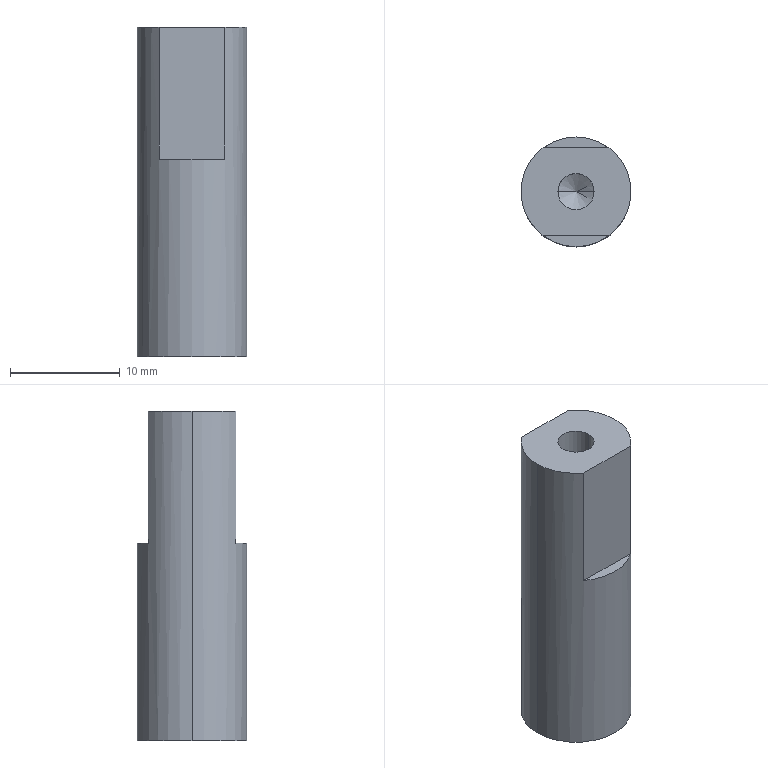Part | STEP file | 2073 Stop shaft | 1 solid | 16 faces | box 10 x 10 x 30 mm | volume 2056 mm3 | cylinder 6 | plane 6 | cone 4 | commonest cylinder face diameters 3.3 x4 10 x2
STEP:
#1=CARTESIAN_POINT('',(0.,0.,0.));
#2=DIRECTION('',(0.,0.,1.));
#3=DIRECTION('',(1.,0.,0.));
#4=AXIS2_PLACEMENT_3D('',#1,#2,#3);
#5=CARTESIAN_POINT('',(-1.65,0.,11.5));
#6=VERTEX_POINT('',#5);
#7=CARTESIAN_POINT('',(-1.65,0.,0.));
#8=VERTEX_POINT('',#7);
#9=CARTESIAN_POINT('',(-1.65,0.,0.));
#10=DIRECTION('',(0.,0.,-1.));
#11=VECTOR('',#10,1.);
#12=LINE('',#9,#11);
#13=CARTESIAN_POINT('',(0.,0.,0.));
#14=DIRECTION('',(0.,0.,-1.));
#15=DIRECTION('',(-1.,0.,0.));
#16=AXIS2_PLACEMENT_3D('',#13,#14,#15);
#17=CYLINDRICAL_SURFACE('',#16,1.65);
#18=CARTESIAN_POINT('',(6.283,0.));
#19=DIRECTION('',(0.,1.));
#20=VECTOR('',#19,1.);
#21=LINE('',#18,#20);
#22=(GEOMETRIC_REPRESENTATION_CONTEXT(2)PARAMETRIC_REPRESENTATION_CONTEXT()REPRESENTATION_CONTEXT('',''));
#23=DEFINITIONAL_REPRESENTATION('',(#21),#22);
#24=PCURVE('',#17,#23);
#25=CARTESIAN_POINT('',(0.,0.,0.));
#26=DIRECTION('',(0.,0.,-1.));
#27=DIRECTION('',(-1.,0.,0.));
#28=AXIS2_PLACEMENT_3D('',#25,#26,#27);
#29=CYLINDRICAL_SURFACE('',#28,1.65);
#30=CARTESIAN_POINT('',(0.,0.));
#31=DIRECTION('',(0.,1.));
#32=VECTOR('',#31,1.);
#33=LINE('',#30,#32);
#34=(GEOMETRIC_REPRESENTATION_CONTEXT(2)PARAMETRIC_REPRESENTATION_CONTEXT()REPRESENTATION_CONTEXT('',''));
#35=DEFINITIONAL_REPRESENTATION('',(#33),#34);
#36=PCURVE('',#29,#35);
#37=SURFACE_CURVE('',#12,(#24,#36),.PCURVE_S1.);
#38=EDGE_CURVE('',#6,#8,#37,.T.);
#39=ORIENTED_EDGE('',*,*,#38,.T.);
#40=CARTESIAN_POINT('',(1.65,0.,0.));
#41=VERTEX_POINT('',#40);
#42=CARTESIAN_POINT('',(0.,0.,0.));
#43=DIRECTION('',(0.,0.,-1.));
#44=DIRECTION('',(-1.,0.,0.));
#45=AXIS2_PLACEMENT_3D('',#42,#43,#44);
#46=CIRCLE('',#45,1.65);
#47=CARTESIAN_POINT('',(0.,0.));
#48=DIRECTION('',(1.,0.));
#49=VECTOR('',#48,1.);
#50=LINE('',#47,#49);
#51=(GEOMETRIC_REPRESENTATION_CONTEXT(2)PARAMETRIC_REPRESENTATION_CONTEXT()REPRESENTATION_CONTEXT('',''));
#52=DEFINITIONAL_REPRESENTATION('',(#50),#51);
#53=PCURVE('',#17,#52);
#54=CARTESIAN_POINT('',(0.,0.,0.));
#55=DIRECTION('',(0.,0.,1.));
#56=DIRECTION('',(1.,0.,0.));
#57=AXIS2_PLACEMENT_3D('',#54,#55,#56);
#58=PLANE('',#57);
#59=CARTESIAN_POINT('',(-1.65,0.));
#60=CARTESIAN_POINT('',(-1.65,2.858));
#61=CARTESIAN_POINT('',(0.825,1.429));
#62=CARTESIAN_POINT('',(3.3,0.));
#63=CARTESIAN_POINT('',(0.825,-1.429));
#64=CARTESIAN_POINT('',(-1.65,-2.858));
#65=CARTESIAN_POINT('',(-1.65,0.));
#66=(BOUNDED_CURVE()B_SPLINE_CURVE(2,(#59,#60,#61,#62,#63,#64,#65),.UNSPECIFIED.,.T.,.F.)B_SPLINE_CURVE_WITH_KNOTS((1,2,2,2,2,1),(-2.094,0.,2.094,4.189,6.283,8.378),.UNSPECIFIED.)CURVE()GEOMETRIC_REPRESENTATION_ITEM()RATIONAL_B_SPLINE_CURVE((1.,0.5,1.,0.5,1.,0.5,1.))REPRESENTATION_ITEM(''));
#67=(GEOMETRIC_REPRESENTATION_CONTEXT(2)PARAMETRIC_REPRESENTATION_CONTEXT()REPRESENTATION_CONTEXT('',''));
#68=DEFINITIONAL_REPRESENTATION('',(#66),#67);
#69=PCURVE('',#58,#68);
#70=SURFACE_CURVE('',#46,(#53,#69),.PCURVE_S1.);
#71=EDGE_CURVE('',#41,#8,#70,.T.);
#72=ORIENTED_EDGE('',*,*,#71,.F.);
#73=CARTESIAN_POINT('',(1.65,0.,11.5));
#74=VERTEX_POINT('',#73);
#75=CARTESIAN_POINT('',(1.65,0.,0.));
#76=DIRECTION('',(0.,0.,-1.));
#77=VECTOR('',#76,1.);
#78=LINE('',#75,#77);
#79=CARTESIAN_POINT('',(3.142,0.));
#80=DIRECTION('',(0.,1.));
#81=VECTOR('',#80,1.);
#82=LINE('',#79,#81);
#83=(GEOMETRIC_REPRESENTATION_CONTEXT(2)PARAMETRIC_REPRESENTATION_CONTEXT()REPRESENTATION_CONTEXT('',''));
#84=DEFINITIONAL_REPRESENTATION('',(#82),#83);
#85=PCURVE('',#17,#84);
#86=CARTESIAN_POINT('',(3.142,0.));
#87=DIRECTION('',(0.,1.));
#88=VECTOR('',#87,1.);
#89=LINE('',#86,#88);
#90=(GEOMETRIC_REPRESENTATION_CONTEXT(2)PARAMETRIC_REPRESENTATION_CONTEXT()REPRESENTATION_CONTEXT('',''));
#91=DEFINITIONAL_REPRESENTATION('',(#89),#90);
#92=PCURVE('',#29,#91);
#93=SURFACE_CURVE('',#78,(#85,#92),.PCURVE_S1.);
#94=EDGE_CURVE('',#74,#41,#93,.T.);
#95=ORIENTED_EDGE('',*,*,#94,.F.);
#96=CARTESIAN_POINT('',(0.,0.,11.5));
#97=DIRECTION('',(0.,0.,-1.));
#98=DIRECTION('',(-1.,0.,0.));
#99=AXIS2_PLACEMENT_3D('',#96,#97,#98);
#100=CIRCLE('',#99,1.65);
#101=CARTESIAN_POINT('',(0.,-11.5));
#102=DIRECTION('',(1.,0.));
#103=VECTOR('',#102,1.);
#104=LINE('',#101,#103);
#105=(GEOMETRIC_REPRESENTATION_CONTEXT(2)PARAMETRIC_REPRESENTATION_CONTEXT()REPRESENTATION_CONTEXT('',''));
#106=DEFINITIONAL_REPRESENTATION('',(#104),#105);
#107=PCURVE('',#17,#106);
#108=CARTESIAN_POINT('',(0.,0.,11.5));
#109=DIRECTION('',(0.,0.,-1.));
#110=DIRECTION('',(-1.,0.,0.));
#111=AXIS2_PLACEMENT_3D('',#108,#109,#110);
#112=CONICAL_SURFACE('',#111,1.65,1.03);
#113=CARTESIAN_POINT('',(0.,0.));
#114=DIRECTION('',(1.,0.));
#115=VECTOR('',#114,1.);
#116=LINE('',#113,#115);
#117=(GEOMETRIC_REPRESENTATION_CONTEXT(2)PARAMETRIC_REPRESENTATION_CONTEXT()REPRESENTATION_CONTEXT('',''));
#118=DEFINITIONAL_REPRESENTATION('',(#116),#117);
#119=PCURVE('',#112,#118);
#120=SURFACE_CURVE('',#100,(#107,#119),.PCURVE_S1.);
#121=EDGE_CURVE('',#74,#6,#120,.T.);
#122=ORIENTED_EDGE('',*,*,#121,.T.);
#123=EDGE_LOOP('',(#39,#72,#95,#122));
#124=FACE_BOUND('',#123,.F.);
#125=ADVANCED_FACE('',(#124),#17,.F.);
#126=ORIENTED_EDGE('',*,*,#121,.F.);
#127=CARTESIAN_POINT('',(0.,0.,12.491));
#128=VERTEX_POINT('',#127);
#129=CARTESIAN_POINT('',(1.65,0.,11.5));
#130=DIRECTION('',(0.8572,0.,-0.515));
#131=VECTOR('',#130,1.);
#132=LINE('',#129,#131);
#133=CARTESIAN_POINT('',(3.142,0.));
#134=DIRECTION('',(0.,1.));
#135=VECTOR('',#134,1.);
#136=LINE('',#133,#135);
#137=(GEOMETRIC_REPRESENTATION_CONTEXT(2)PARAMETRIC_REPRESENTATION_CONTEXT()REPRESENTATION_CONTEXT('',''));
#138=DEFINITIONAL_REPRESENTATION('',(#136),#137);
#139=PCURVE('',#112,#138);
#140=CARTESIAN_POINT('',(0.,0.,11.5));
#141=DIRECTION('',(0.,0.,-1.));
#142=DIRECTION('',(-1.,0.,0.));
#143=AXIS2_PLACEMENT_3D('',#140,#141,#142);
#144=CONICAL_SURFACE('',#143,1.65,1.03);
#145=CARTESIAN_POINT('',(3.142,0.));
#146=DIRECTION('',(0.,1.));
#147=VECTOR('',#146,1.);
#148=LINE('',#145,#147);
#149=(GEOMETRIC_REPRESENTATION_CONTEXT(2)PARAMETRIC_REPRESENTATION_CONTEXT()REPRESENTATION_CONTEXT('',''));
#150=DEFINITIONAL_REPRESENTATION('',(#148),#149);
#151=PCURVE('',#144,#150);
#152=SURFACE_CURVE('',#132,(#139,#151),.PCURVE_S1.);
#153=EDGE_CURVE('',#128,#74,#152,.T.);
#154=ORIENTED_EDGE('',*,*,#153,.F.);
#155=CARTESIAN_POINT('',(-1.65,0.,11.5));
#156=DIRECTION('',(-0.8572,0.,-0.515));
#157=VECTOR('',#156,1.);
#158=LINE('',#155,#157);
#159=CARTESIAN_POINT('',(6.283,0.));
#160=DIRECTION('',(0.,1.));
#161=VECTOR('',#160,1.);
#162=LINE('',#159,#161);
#163=(GEOMETRIC_REPRESENTATION_CONTEXT(2)PARAMETRIC_REPRESENTATION_CONTEXT()REPRESENTATION_CONTEXT('',''));
#164=DEFINITIONAL_REPRESENTATION('',(#162),#163);
#165=PCURVE('',#112,#164);
#166=CARTESIAN_POINT('',(0.,0.));
#167=DIRECTION('',(0.,1.));
#168=VECTOR('',#167,1.);
#169=LINE('',#166,#168);
#170=(GEOMETRIC_REPRESENTATION_CONTEXT(2)PARAMETRIC_REPRESENTATION_CONTEXT()REPRESENTATION_CONTEXT('',''));
#171=DEFINITIONAL_REPRESENTATION('',(#169),#170);
#172=PCURVE('',#144,#171);
#173=SURFACE_CURVE('',#158,(#165,#172),.PCURVE_S1.);
#174=EDGE_CURVE('',#128,#6,#173,.T.);
#175=ORIENTED_EDGE('',*,*,#174,.T.);
#176=EDGE_LOOP('',(#126,#154,#175));
#177=FACE_BOUND('',#176,.F.);
#178=ADVANCED_FACE('',(#177),#112,.F.);
#179=CARTESIAN_POINT('',(1.65,0.,18.5));
#180=VERTEX_POINT('',#179);
#181=CARTESIAN_POINT('',(1.65,0.,30.));
#182=VERTEX_POINT('',#181);
#183=CARTESIAN_POINT('',(1.65,0.,30.));
#184=DIRECTION('',(0.,0.,1.));
#185=VECTOR('',#184,1.);
#186=LINE('',#183,#185);
#187=CARTESIAN_POINT('',(0.,0.,30.));
#188=DIRECTION('',(0.,0.,1.));
#189=DIRECTION('',(1.,0.,0.));
#190=AXIS2_PLACEMENT_3D('',#187,#188,#189);
#191=CYLINDRICAL_SURFACE('',#190,1.65);
#192=CARTESIAN_POINT('',(6.283,0.));
#193=DIRECTION('',(0.,1.));
#194=VECTOR('',#193,1.);
#195=LINE('',#192,#194);
#196=(GEOMETRIC_REPRESENTATION_CONTEXT(2)PARAMETRIC_REPRESENTATION_CONTEXT()REPRESENTATION_CONTEXT('',''));
#197=DEFINITIONAL_REPRESENTATION('',(#195),#196);
#198=PCURVE('',#191,#197);
#199=CARTESIAN_POINT('',(0.,0.,30.));
#200=DIRECTION('',(0.,0.,1.));
#201=DIRECTION('',(1.,0.,0.));
#202=AXIS2_PLACEMENT_3D('',#199,#200,#201);
#203=CYLINDRICAL_SURFACE('',#202,1.65);
#204=CARTESIAN_POINT('',(0.,0.));
#205=DIRECTION('',(0.,1.));
#206=VECTOR('',#205,1.);
#207=LINE('',#204,#206);
#208=(GEOMETRIC_REPRESENTATION_CONTEXT(2)PARAMETRIC_REPRESENTATION_CONTEXT()REPRESENTATION_CONTEXT('',''));
#209=DEFINITIONAL_REPRESENTATION('',(#207),#208);
#210=PCURVE('',#203,#209);
#211=SURFACE_CURVE('',#186,(#198,#210),.PCURVE_S1.);
#212=EDGE_CURVE('',#180,#182,#211,.T.);
#213=ORIENTED_EDGE('',*,*,#212,.T.);
#214=CARTESIAN_POINT('',(-1.65,0.,30.));
#215=VERTEX_POINT('',#214);
#216=CARTESIAN_POINT('',(0.,0.,30.));
#217=DIRECTION('',(0.,0.,1.));
#218=DIRECTION('',(1.,0.,0.));
#219=AXIS2_PLACEMENT_3D('',#216,#217,#218);
#220=CIRCLE('',#219,1.65);
#221=CARTESIAN_POINT('',(0.,0.));
#222=DIRECTION('',(1.,0.));
#223=VECTOR('',#222,1.);
#224=LINE('',#221,#223);
#225=(GEOMETRIC_REPRESENTATION_CONTEXT(2)PARAMETRIC_REPRESENTATION_CONTEXT()REPRESENTATION_CONTEXT('',''));
#226=DEFINITIONAL_REPRESENTATION('',(#224),#225);
#227=PCURVE('',#191,#226);
#228=CARTESIAN_POINT('',(0.,0.,30.));
#229=DIRECTION('',(0.,0.,1.));
#230=DIRECTION('',(1.,0.,0.));
#231=AXIS2_PLACEMENT_3D('',#228,#229,#230);
#232=PLANE('',#231);
#233=CARTESIAN_POINT('',(0.,0.));
#234=DIRECTION('',(1.,0.));
#235=AXIS2_PLACEMENT_2D('',#233,#234);
#236=CIRCLE('',#235,1.65);
#237=(GEOMETRIC_REPRESENTATION_CONTEXT(2)PARAMETRIC_REPRESENTATION_CONTEXT()REPRESENTATION_CONTEXT('',''));
#238=DEFINITIONAL_REPRESENTATION('',(#236),#237);
#239=PCURVE('',#232,#238);
#240=SURFACE_CURVE('',#220,(#227,#239),.PCURVE_S1.);
#241=EDGE_CURVE('',#215,#182,#240,.T.);
#242=ORIENTED_EDGE('',*,*,#241,.F.);
#243=CARTESIAN_POINT('',(-1.65,0.,18.5));
#244=VERTEX_POINT('',#243);
#245=CARTESIAN_POINT('',(-1.65,0.,30.));
#246=DIRECTION('',(0.,0.,1.));
#247=VECTOR('',#246,1.);
#248=LINE('',#245,#247);
#249=CARTESIAN_POINT('',(3.142,0.));
#250=DIRECTION('',(0.,1.));
#251=VECTOR('',#250,1.);
#252=LINE('',#249,#251);
#253=(GEOMETRIC_REPRESENTATION_CONTEXT(2)PARAMETRIC_REPRESENTATION_CONTEXT()REPRESENTATION_CONTEXT('',''));
#254=DEFINITIONAL_REPRESENTATION('',(#252),#253);
#255=PCURVE('',#191,#254);
#256=CARTESIAN_POINT('',(3.142,0.));
#257=DIRECTION('',(0.,1.));
#258=VECTOR('',#257,1.);
#259=LINE('',#256,#258);
#260=(GEOMETRIC_REPRESENTATION_CONTEXT(2)PARAMETRIC_REPRESENTATION_CONTEXT()REPRESENTATION_CONTEXT('',''));
#261=DEFINITIONAL_REPRESENTATION('',(#259),#260);
#262=PCURVE('',#203,#261);
#263=SURFACE_CURVE('',#248,(#255,#262),.PCURVE_S1.);
#264=EDGE_CURVE('',#244,#215,#263,.T.);
#265=ORIENTED_EDGE('',*,*,#264,.F.);
#266=CARTESIAN_POINT('',(0.,0.,18.5));
#267=DIRECTION('',(0.,0.,1.));
#268=DIRECTION('',(1.,0.,0.));
#269=AXIS2_PLACEMENT_3D('',#266,#267,#268);
#270=CIRCLE('',#269,1.65);
#271=CARTESIAN_POINT('',(0.,-11.5));
#272=DIRECTION('',(1.,0.));
#273=VECTOR('',#272,1.);
#274=LINE('',#271,#273);
#275=(GEOMETRIC_REPRESENTATION_CONTEXT(2)PARAMETRIC_REPRESENTATION_CONTEXT()REPRESENTATION_CONTEXT('',''));
#276=DEFINITIONAL_REPRESENTATION('',(#274),#275);
#277=PCURVE('',#191,#276);
#278=CARTESIAN_POINT('',(0.,0.,18.5));
#279=DIRECTION('',(0.,0.,1.));
#280=DIRECTION('',(1.,0.,0.));
#281=AXIS2_PLACEMENT_3D('',#278,#279,#280);
#282=CONICAL_SURFACE('',#281,1.65,1.03);
#283=CARTESIAN_POINT('',(0.,0.));
#284=DIRECTION('',(1.,0.));
#285=VECTOR('',#284,1.);
#286=LINE('',#283,#285);
#287=(GEOMETRIC_REPRESENTATION_CONTEXT(2)PARAMETRIC_REPRESENTATION_CONTEXT()REPRESENTATION_CONTEXT('',''));
#288=DEFINITIONAL_REPRESENTATION('',(#286),#287);
#289=PCURVE('',#282,#288);
#290=SURFACE_CURVE('',#270,(#277,#289),.PCURVE_S1.);
#291=EDGE_CURVE('',#244,#180,#290,.T.);
#292=ORIENTED_EDGE('',*,*,#291,.T.);
#293=EDGE_LOOP('',(#213,#242,#265,#292));
#294=FACE_BOUND('',#293,.F.);
#295=ADVANCED_FACE('',(#294),#191,.F.);
#296=ORIENTED_EDGE('',*,*,#291,.F.);
#297=CARTESIAN_POINT('',(0.,0.,17.509));
#298=VERTEX_POINT('',#297);
#299=CARTESIAN_POINT('',(-1.65,0.,18.5));
#300=DIRECTION('',(-0.8572,0.,0.515));
#301=VECTOR('',#300,1.);
#302=LINE('',#299,#301);
#303=CARTESIAN_POINT('',(3.142,0.));
#304=DIRECTION('',(0.,1.));
#305=VECTOR('',#304,1.);
#306=LINE('',#303,#305);
#307=(GEOMETRIC_REPRESENTATION_CONTEXT(2)PARAMETRIC_REPRESENTATION_CONTEXT()REPRESENTATION_CONTEXT('',''));
#308=DEFINITIONAL_REPRESENTATION('',(#306),#307);
#309=PCURVE('',#282,#308);
#310=CARTESIAN_POINT('',(0.,0.,18.5));
#311=DIRECTION('',(0.,0.,1.));
#312=DIRECTION('',(1.,0.,0.));
#313=AXIS2_PLACEMENT_3D('',#310,#311,#312);
#314=CONICAL_SURFACE('',#313,1.65,1.03);
#315=CARTESIAN_POINT('',(3.142,0.));
#316=DIRECTION('',(0.,1.));
#317=VECTOR('',#316,1.);
#318=LINE('',#315,#317);
#319=(GEOMETRIC_REPRESENTATION_CONTEXT(2)PARAMETRIC_REPRESENTATION_CONTEXT()REPRESENTATION_CONTEXT('',''));
#320=DEFINITIONAL_REPRESENTATION('',(#318),#319);
#321=PCURVE('',#314,#320);
#322=SURFACE_CURVE('',#302,(#309,#321),.PCURVE_S1.);
#323=EDGE_CURVE('',#298,#244,#322,.T.);
#324=ORIENTED_EDGE('',*,*,#323,.F.);
#325=CARTESIAN_POINT('',(1.65,0.,18.5));
#326=DIRECTION('',(0.8572,0.,0.515));
#327=VECTOR('',#326,1.);
#328=LINE('',#325,#327);
#329=CARTESIAN_POINT('',(6.283,-0.9914));
#330=CARTESIAN_POINT('',(6.283,-0.9764));
#331=CARTESIAN_POINT('',(6.283,-0.9464));
#332=CARTESIAN_POINT('',(6.283,-0.9013));
#333=CARTESIAN_POINT('',(6.283,-0.8562));
#334=CARTESIAN_POINT('',(6.283,-0.8112));
#335=CARTESIAN_POINT('',(6.283,-0.7661));
#336=CARTESIAN_POINT('',(6.283,-0.721));
#337=CARTESIAN_POINT('',(6.283,-0.676));
#338=CARTESIAN_POINT('',(6.283,-0.6309));
#339=CARTESIAN_POINT('',(6.283,-0.5858));
#340=CARTESIAN_POINT('',(6.283,-0.5408));
#341=CARTESIAN_POINT('',(6.283,-0.4957));
#342=CARTESIAN_POINT('',(6.283,-0.4506));
#343=CARTESIAN_POINT('',(6.283,-0.4056));
#344=CARTESIAN_POINT('',(6.283,-0.3605));
#345=CARTESIAN_POINT('',(6.283,-0.3155));
#346=CARTESIAN_POINT('',(6.283,-0.2704));
#347=CARTESIAN_POINT('',(6.283,-0.2253));
#348=CARTESIAN_POINT('',(6.283,-0.1803));
#349=CARTESIAN_POINT('',(6.283,-0.1352));
#350=CARTESIAN_POINT('',(6.283,-0.09013));
#351=CARTESIAN_POINT('',(6.283,-0.04506));
#352=CARTESIAN_POINT('',(6.283,-0.01502));
#353=CARTESIAN_POINT('',(6.283,0.));
#354=B_SPLINE_CURVE_WITH_KNOTS('',3,(#329,#330,#331,#332,#333,#334,#335,#336,#337,#338,#339,#340,#341,#342,#343,#344,#345,#346,#347,#348,#349,#350,#351,#352,#353),.UNSPECIFIED.,.F.,.F.,(4,1,1,1,1,1,1,1,1,1,1,1,1,1,1,1,1,1,1,1,1,1,4),(-1.925,-1.837,-1.75,-1.662,-1.575,-1.487,-1.4,-1.312,-1.225,-1.137,-1.05,-0.9625,-0.875,-0.7875,-0.7,-0.6125,-0.525,-0.4375,-0.35,-0.2625,-0.175,-0.0875,0.),.UNSPECIFIED.);
#355=(GEOMETRIC_REPRESENTATION_CONTEXT(2)PARAMETRIC_REPRESENTATION_CONTEXT()REPRESENTATION_CONTEXT('',''));
#356=DEFINITIONAL_REPRESENTATION('',(#354),#355);
#357=PCURVE('',#282,#356);
#358=CARTESIAN_POINT('',(0.,-0.9914));
#359=CARTESIAN_POINT('',(0.,-0.9764));
#360=CARTESIAN_POINT('',(0.,-0.9464));
#361=CARTESIAN_POINT('',(0.,-0.9013));
#362=CARTESIAN_POINT('',(0.,-0.8562));
#363=CARTESIAN_POINT('',(0.,-0.8112));
#364=CARTESIAN_POINT('',(0.,-0.7661));
#365=CARTESIAN_POINT('',(0.,-0.721));
#366=CARTESIAN_POINT('',(0.,-0.676));
#367=CARTESIAN_POINT('',(0.,-0.6309));
#368=CARTESIAN_POINT('',(0.,-0.5858));
#369=CARTESIAN_POINT('',(0.,-0.5408));
#370=CARTESIAN_POINT('',(0.,-0.4957));
#371=CARTESIAN_POINT('',(0.,-0.4506));
#372=CARTESIAN_POINT('',(0.,-0.4056));
#373=CARTESIAN_POINT('',(0.,-0.3605));
#374=CARTESIAN_POINT('',(0.,-0.3155));
#375=CARTESIAN_POINT('',(0.,-0.2704));
#376=CARTESIAN_POINT('',(0.,-0.2253));
#377=CARTESIAN_POINT('',(0.,-0.1803));
#378=CARTESIAN_POINT('',(0.,-0.1352));
#379=CARTESIAN_POINT('',(0.,-0.09013));
#380=CARTESIAN_POINT('',(0.,-0.04506));
#381=CARTESIAN_POINT('',(0.,-0.01502));
#382=CARTESIAN_POINT('',(0.,0.));
#383=B_SPLINE_CURVE_WITH_KNOTS('',3,(#358,#359,#360,#361,#362,#363,#364,#365,#366,#367,#368,#369,#370,#371,#372,#373,#374,#375,#376,#377,#378,#379,#380,#381,#382),.UNSPECIFIED.,.F.,.F.,(4,1,1,1,1,1,1,1,1,1,1,1,1,1,1,1,1,1,1,1,1,1,4),(-1.925,-1.837,-1.75,-1.662,-1.575,-1.487,-1.4,-1.312,-1.225,-1.137,-1.05,-0.9625,-0.875,-0.7875,-0.7,-0.6125,-0.525,-0.4375,-0.35,-0.2625,-0.175,-0.0875,0.),.UNSPECIFIED.);
#384=(GEOMETRIC_REPRESENTATION_CONTEXT(2)PARAMETRIC_REPRESENTATION_CONTEXT()REPRESENTATION_CONTEXT('',''));
#385=DEFINITIONAL_REPRESENTATION('',(#383),#384);
#386=PCURVE('',#314,#385);
#387=SURFACE_CURVE('',#328,(#357,#386),.PCURVE_S1.);
#388=EDGE_CURVE('',#298,#180,#387,.T.);
#389=ORIENTED_EDGE('',*,*,#388,.T.);
#390=EDGE_LOOP('',(#296,#324,#389));
#391=FACE_BOUND('',#390,.F.);
#392=ADVANCED_FACE('',(#391),#282,.F.);
#393=CARTESIAN_POINT('',(5.,0.,30.));
#394=VERTEX_POINT('',#393);
#395=CARTESIAN_POINT('',(3.,4.,30.));
#396=VERTEX_POINT('',#395);
#397=CARTESIAN_POINT('',(0.,0.,30.));
#398=DIRECTION('',(0.,0.,1.));
#399=DIRECTION('',(1.,0.,0.));
#400=AXIS2_PLACEMENT_3D('',#397,#398,#399);
#401=CIRCLE('',#400,5.);
#402=CARTESIAN_POINT('',(0.,0.,30.));
#403=DIRECTION('',(0.,0.,-1.));
#404=DIRECTION('',(-1.,0.,0.));
#405=AXIS2_PLACEMENT_3D('',#402,#403,#404);
#406=CYLINDRICAL_SURFACE('',#405,5.);
#407=CARTESIAN_POINT('',(3.142,0.));
#408=DIRECTION('',(-1.,0.));
#409=VECTOR('',#408,1.);
#410=LINE('',#407,#409);
#411=(GEOMETRIC_REPRESENTATION_CONTEXT(2)PARAMETRIC_REPRESENTATION_CONTEXT()REPRESENTATION_CONTEXT('',''));
#412=DEFINITIONAL_REPRESENTATION('',(#410),#411);
#413=PCURVE('',#406,#412);
#414=CARTESIAN_POINT('',(0.,0.));
#415=DIRECTION('',(1.,0.));
#416=AXIS2_PLACEMENT_2D('',#414,#415);
#417=CIRCLE('',#416,5.);
#418=(GEOMETRIC_REPRESENTATION_CONTEXT(2)PARAMETRIC_REPRESENTATION_CONTEXT()REPRESENTATION_CONTEXT('',''));
#419=DEFINITIONAL_REPRESENTATION('',(#417),#418);
#420=PCURVE('',#232,#419);
#421=SURFACE_CURVE('',#401,(#413,#420),.PCURVE_S1.);
#422=EDGE_CURVE('',#394,#396,#421,.T.);
#423=ORIENTED_EDGE('',*,*,#422,.F.);
#424=CARTESIAN_POINT('',(5.,0.,0.));
#425=VERTEX_POINT('',#424);
#426=CARTESIAN_POINT('',(5.,0.,30.));
#427=DIRECTION('',(0.,0.,-1.));
#428=VECTOR('',#427,1.);
#429=LINE('',#426,#428);
#430=CARTESIAN_POINT('',(3.142,0.));
#431=DIRECTION('',(0.,1.));
#432=VECTOR('',#431,1.);
#433=LINE('',#430,#432);
#434=(GEOMETRIC_REPRESENTATION_CONTEXT(2)PARAMETRIC_REPRESENTATION_CONTEXT()REPRESENTATION_CONTEXT('',''));
#435=DEFINITIONAL_REPRESENTATION('',(#433),#434);
#436=PCURVE('',#406,#435);
#437=CARTESIAN_POINT('',(0.,0.,30.));
#438=DIRECTION('',(0.,0.,-1.));
#439=DIRECTION('',(-1.,0.,0.));
#440=AXIS2_PLACEMENT_3D('',#437,#438,#439);
#441=CYLINDRICAL_SURFACE('',#440,5.);
#442=CARTESIAN_POINT('',(3.142,0.));
#443=DIRECTION('',(0.,1.));
#444=VECTOR('',#443,1.);
#445=LINE('',#442,#444);
#446=(GEOMETRIC_REPRESENTATION_CONTEXT(2)PARAMETRIC_REPRESENTATION_CONTEXT()REPRESENTATION_CONTEXT('',''));
#447=DEFINITIONAL_REPRESENTATION('',(#445),#446);
#448=PCURVE('',#441,#447);
#449=SURFACE_CURVE('',#429,(#436,#448),.PCURVE_S1.);
#450=EDGE_CURVE('',#394,#425,#449,.T.);
#451=ORIENTED_EDGE('',*,*,#450,.T.);
#452=CARTESIAN_POINT('',(-5.,0.,0.));
#453=VERTEX_POINT('',#452);
#454=CARTESIAN_POINT('',(0.,0.,0.));
#455=DIRECTION('',(0.,0.,1.));
#456=DIRECTION('',(1.,0.,0.));
#457=AXIS2_PLACEMENT_3D('',#454,#455,#456);
#458=CIRCLE('',#457,5.);
#459=CARTESIAN_POINT('',(3.142,30.));
#460=DIRECTION('',(-1.,0.));
#461=VECTOR('',#460,1.);
#462=LINE('',#459,#461);
#463=(GEOMETRIC_REPRESENTATION_CONTEXT(2)PARAMETRIC_REPRESENTATION_CONTEXT()REPRESENTATION_CONTEXT('',''));
#464=DEFINITIONAL_REPRESENTATION('',(#462),#463);
#465=PCURVE('',#406,#464);
#466=CARTESIAN_POINT('',(0.,0.));
#467=DIRECTION('',(1.,0.));
#468=AXIS2_PLACEMENT_2D('',#466,#467);
#469=CIRCLE('',#468,5.);
#470=(GEOMETRIC_REPRESENTATION_CONTEXT(2)PARAMETRIC_REPRESENTATION_CONTEXT()REPRESENTATION_CONTEXT('',''));
#471=DEFINITIONAL_REPRESENTATION('',(#469),#470);
#472=PCURVE('',#58,#471);
#473=SURFACE_CURVE('',#458,(#465,#472),.PCURVE_S1.);
#474=EDGE_CURVE('',#425,#453,#473,.T.);
#475=ORIENTED_EDGE('',*,*,#474,.T.);
#476=CARTESIAN_POINT('',(-5.,0.,30.));
#477=VERTEX_POINT('',#476);
#478=CARTESIAN_POINT('',(-5.,0.,30.));
#479=DIRECTION('',(0.,0.,-1.));
#480=VECTOR('',#479,1.);
#481=LINE('',#478,#480);
#482=CARTESIAN_POINT('',(0.,0.));
#483=DIRECTION('',(0.,1.));
#484=VECTOR('',#483,1.);
#485=LINE('',#482,#484);
#486=(GEOMETRIC_REPRESENTATION_CONTEXT(2)PARAMETRIC_REPRESENTATION_CONTEXT()REPRESENTATION_CONTEXT('',''));
#487=DEFINITIONAL_REPRESENTATION('',(#485),#486);
#488=PCURVE('',#406,#487);
#489=CARTESIAN_POINT('',(6.283,0.));
#490=DIRECTION('',(0.,1.));
#491=VECTOR('',#490,1.);
#492=LINE('',#489,#491);
#493=(GEOMETRIC_REPRESENTATION_CONTEXT(2)PARAMETRIC_REPRESENTATION_CONTEXT()REPRESENTATION_CONTEXT('',''));
#494=DEFINITIONAL_REPRESENTATION('',(#492),#493);
#495=PCURVE('',#441,#494);
#496=SURFACE_CURVE('',#481,(#488,#495),.PCURVE_S1.);
#497=EDGE_CURVE('',#477,#453,#496,.T.);
#498=ORIENTED_EDGE('',*,*,#497,.F.);
#499=CARTESIAN_POINT('',(-3.,4.,30.));
#500=VERTEX_POINT('',#499);
#501=CARTESIAN_POINT('',(0.,0.,30.));
#502=DIRECTION('',(0.,0.,1.));
#503=DIRECTION('',(1.,0.,0.));
#504=AXIS2_PLACEMENT_3D('',#501,#502,#503);
#505=CIRCLE('',#504,5.);
#506=CARTESIAN_POINT('',(3.142,0.));
#507=DIRECTION('',(-1.,0.));
#508=VECTOR('',#507,1.);
#509=LINE('',#506,#508);
#510=(GEOMETRIC_REPRESENTATION_CONTEXT(2)PARAMETRIC_REPRESENTATION_CONTEXT()REPRESENTATION_CONTEXT('',''));
#511=DEFINITIONAL_REPRESENTATION('',(#509),#510);
#512=PCURVE('',#406,#511);
#513=CARTESIAN_POINT('',(0.,0.));
#514=DIRECTION('',(1.,0.));
#515=AXIS2_PLACEMENT_2D('',#513,#514);
#516=CIRCLE('',#515,5.);
#517=(GEOMETRIC_REPRESENTATION_CONTEXT(2)PARAMETRIC_REPRESENTATION_CONTEXT()REPRESENTATION_CONTEXT('',''));
#518=DEFINITIONAL_REPRESENTATION('',(#516),#517);
#519=PCURVE('',#232,#518);
#520=SURFACE_CURVE('',#505,(#512,#519),.PCURVE_S1.);
#521=EDGE_CURVE('',#500,#477,#520,.T.);
#522=ORIENTED_EDGE('',*,*,#521,.F.);
#523=CARTESIAN_POINT('',(-3.,4.,18.));
#524=VERTEX_POINT('',#523);
#525=CARTESIAN_POINT('',(-3.,4.,30.));
#526=DIRECTION('',(0.,0.,-1.));
#527=VECTOR('',#526,1.);
#528=LINE('',#525,#527);
#529=CARTESIAN_POINT('',(0.9273,0.));
#530=DIRECTION('',(0.,1.));
#531=VECTOR('',#530,1.);
#532=LINE('',#529,#531);
#533=(GEOMETRIC_REPRESENTATION_CONTEXT(2)PARAMETRIC_REPRESENTATION_CONTEXT()REPRESENTATION_CONTEXT('',''));
#534=DEFINITIONAL_REPRESENTATION('',(#532),#533);
#535=PCURVE('',#406,#534);
#536=CARTESIAN_POINT('',(-6.568,4.,18.));
#537=DIRECTION('',(0.,-1.,0.));
#538=DIRECTION('',(0.,0.,-1.));
#539=AXIS2_PLACEMENT_3D('',#536,#537,#538);
#540=PLANE('',#539);
#541=CARTESIAN_POINT('',(-12.,3.568));
#542=DIRECTION('',(1.,0.));
#543=VECTOR('',#542,1.);
#544=LINE('',#541,#543);
#545=(GEOMETRIC_REPRESENTATION_CONTEXT(2)PARAMETRIC_REPRESENTATION_CONTEXT()REPRESENTATION_CONTEXT('',''));
#546=DEFINITIONAL_REPRESENTATION('',(#544),#545);
#547=PCURVE('',#540,#546);
#548=SURFACE_CURVE('',#528,(#535,#547),.PCURVE_S1.);
#549=EDGE_CURVE('',#500,#524,#548,.T.);
#550=ORIENTED_EDGE('',*,*,#549,.T.);
#551=CARTESIAN_POINT('',(3.,4.,18.));
#552=VERTEX_POINT('',#551);
#553=CARTESIAN_POINT('',(0.,0.,18.));
#554=DIRECTION('',(0.,0.,1.));
#555=DIRECTION('',(1.,0.,0.));
#556=AXIS2_PLACEMENT_3D('',#553,#554,#555);
#557=CIRCLE('',#556,5.);
#558=CARTESIAN_POINT('',(3.142,12.));
#559=DIRECTION('',(-1.,0.));
#560=VECTOR('',#559,1.);
#561=LINE('',#558,#560);
#562=(GEOMETRIC_REPRESENTATION_CONTEXT(2)PARAMETRIC_REPRESENTATION_CONTEXT()REPRESENTATION_CONTEXT('',''));
#563=DEFINITIONAL_REPRESENTATION('',(#561),#562);
#564=PCURVE('',#406,#563);
#565=CARTESIAN_POINT('',(0.,0.,18.));
#566=DIRECTION('',(0.,0.,1.));
#567=DIRECTION('',(1.,0.,0.));
#568=AXIS2_PLACEMENT_3D('',#565,#566,#567);
#569=PLANE('',#568);
#570=CARTESIAN_POINT('',(0.,0.));
#571=DIRECTION('',(1.,0.));
#572=AXIS2_PLACEMENT_2D('',#570,#571);
#573=CIRCLE('',#572,5.);
#574=(GEOMETRIC_REPRESENTATION_CONTEXT(2)PARAMETRIC_REPRESENTATION_CONTEXT()REPRESENTATION_CONTEXT('',''));
#575=DEFINITIONAL_REPRESENTATION('',(#573),#574);
#576=PCURVE('',#569,#575);
#577=SURFACE_CURVE('',#557,(#564,#576),.PCURVE_S1.);
#578=EDGE_CURVE('',#552,#524,#577,.T.);
#579=ORIENTED_EDGE('',*,*,#578,.F.);
#580=CARTESIAN_POINT('',(3.,4.,30.));
#581=DIRECTION('',(0.,0.,1.));
#582=VECTOR('',#581,1.);
#583=LINE('',#580,#582);
#584=CARTESIAN_POINT('',(2.214,0.));
#585=DIRECTION('',(0.,-1.));
#586=VECTOR('',#585,1.);
#587=LINE('',#584,#586);
#588=(GEOMETRIC_REPRESENTATION_CONTEXT(2)PARAMETRIC_REPRESENTATION_CONTEXT()REPRESENTATION_CONTEXT('',''));
#589=DEFINITIONAL_REPRESENTATION('',(#587),#588);
#590=PCURVE('',#406,#589);
#591=CARTESIAN_POINT('',(-12.,9.568));
#592=DIRECTION('',(-1.,0.));
#593=VECTOR('',#592,1.);
#594=LINE('',#591,#593);
#595=(GEOMETRIC_REPRESENTATION_CONTEXT(2)PARAMETRIC_REPRESENTATION_CONTEXT()REPRESENTATION_CONTEXT('',''));
#596=DEFINITIONAL_REPRESENTATION('',(#594),#595);
#597=PCURVE('',#540,#596);
#598=SURFACE_CURVE('',#583,(#590,#597),.PCURVE_S1.);
#599=EDGE_CURVE('',#552,#396,#598,.T.);
#600=ORIENTED_EDGE('',*,*,#599,.T.);
#601=EDGE_LOOP('',(#423,#451,#475,#498,#522,#550,#579,#600));
#602=FACE_BOUND('',#601,.T.);
#603=ADVANCED_FACE('',(#602),#406,.T.);
#604=ORIENTED_EDGE('',*,*,#450,.F.);
#605=CARTESIAN_POINT('',(3.,-4.,30.));
#606=VERTEX_POINT('',#605);
#607=CARTESIAN_POINT('',(0.,0.,30.));
#608=DIRECTION('',(0.,0.,1.));
#609=DIRECTION('',(1.,0.,0.));
#610=AXIS2_PLACEMENT_3D('',#607,#608,#609);
#611=CIRCLE('',#610,5.);
#612=CARTESIAN_POINT('',(9.425,0.));
#613=DIRECTION('',(-1.,0.));
#614=VECTOR('',#613,1.);
#615=LINE('',#612,#614);
#616=(GEOMETRIC_REPRESENTATION_CONTEXT(2)PARAMETRIC_REPRESENTATION_CONTEXT()REPRESENTATION_CONTEXT('',''));
#617=DEFINITIONAL_REPRESENTATION('',(#615),#616);
#618=PCURVE('',#441,#617);
#619=CARTESIAN_POINT('',(0.,0.));
#620=DIRECTION('',(1.,0.));
#621=AXIS2_PLACEMENT_2D('',#619,#620);
#622=CIRCLE('',#621,5.);
#623=(GEOMETRIC_REPRESENTATION_CONTEXT(2)PARAMETRIC_REPRESENTATION_CONTEXT()REPRESENTATION_CONTEXT('',''));
#624=DEFINITIONAL_REPRESENTATION('',(#622),#623);
#625=PCURVE('',#232,#624);
#626=SURFACE_CURVE('',#611,(#618,#625),.PCURVE_S1.);
#627=EDGE_CURVE('',#606,#394,#626,.T.);
#628=ORIENTED_EDGE('',*,*,#627,.F.);
#629=CARTESIAN_POINT('',(3.,-4.,18.));
#630=VERTEX_POINT('',#629);
#631=CARTESIAN_POINT('',(3.,-4.,30.));
#632=DIRECTION('',(0.,0.,-1.));
#633=VECTOR('',#632,1.);
#634=LINE('',#631,#633);
#635=CARTESIAN_POINT('',(4.069,0.));
#636=DIRECTION('',(0.,1.));
#637=VECTOR('',#636,1.);
#638=LINE('',#635,#637);
#639=(GEOMETRIC_REPRESENTATION_CONTEXT(2)PARAMETRIC_REPRESENTATION_CONTEXT()REPRESENTATION_CONTEXT('',''));
#640=DEFINITIONAL_REPRESENTATION('',(#638),#639);
#641=PCURVE('',#441,#640);
#642=CARTESIAN_POINT('',(-6.782,-4.,18.));
#643=DIRECTION('',(0.,1.,0.));
#644=DIRECTION('',(0.,0.,1.));
#645=AXIS2_PLACEMENT_3D('',#642,#643,#644);
#646=PLANE('',#645);
#647=CARTESIAN_POINT('',(12.,9.782));
#648=DIRECTION('',(-1.,0.));
#649=VECTOR('',#648,1.);
#650=LINE('',#647,#649);
#651=(GEOMETRIC_REPRESENTATION_CONTEXT(2)PARAMETRIC_REPRESENTATION_CONTEXT()REPRESENTATION_CONTEXT('',''));
#652=DEFINITIONAL_REPRESENTATION('',(#650),#651);
#653=PCURVE('',#646,#652);
#654=SURFACE_CURVE('',#634,(#641,#653),.PCURVE_S1.);
#655=EDGE_CURVE('',#606,#630,#654,.T.);
#656=ORIENTED_EDGE('',*,*,#655,.T.);
#657=CARTESIAN_POINT('',(-3.,-4.,18.));
#658=VERTEX_POINT('',#657);
#659=CARTESIAN_POINT('',(0.,0.,18.));
#660=DIRECTION('',(0.,0.,1.));
#661=DIRECTION('',(1.,0.,0.));
#662=AXIS2_PLACEMENT_3D('',#659,#660,#661);
#663=CIRCLE('',#662,5.);
#664=CARTESIAN_POINT('',(9.425,12.));
#665=DIRECTION('',(-1.,0.));
#666=VECTOR('',#665,1.);
#667=LINE('',#664,#666);
#668=(GEOMETRIC_REPRESENTATION_CONTEXT(2)PARAMETRIC_REPRESENTATION_CONTEXT()REPRESENTATION_CONTEXT('',''));
#669=DEFINITIONAL_REPRESENTATION('',(#667),#668);
#670=PCURVE('',#441,#669);
#671=CARTESIAN_POINT('',(0.,0.,18.));
#672=DIRECTION('',(0.,0.,1.));
#673=DIRECTION('',(1.,0.,0.));
#674=AXIS2_PLACEMENT_3D('',#671,#672,#673);
#675=PLANE('',#674);
#676=CARTESIAN_POINT('',(0.,0.));
#677=DIRECTION('',(1.,0.));
#678=AXIS2_PLACEMENT_2D('',#676,#677);
#679=CIRCLE('',#678,5.);
#680=(GEOMETRIC_REPRESENTATION_CONTEXT(2)PARAMETRIC_REPRESENTATION_CONTEXT()REPRESENTATION_CONTEXT('',''));
#681=DEFINITIONAL_REPRESENTATION('',(#679),#680);
#682=PCURVE('',#675,#681);
#683=SURFACE_CURVE('',#663,(#670,#682),.PCURVE_S1.);
#684=EDGE_CURVE('',#658,#630,#683,.T.);
#685=ORIENTED_EDGE('',*,*,#684,.F.);
#686=CARTESIAN_POINT('',(-3.,-4.,30.));
#687=VERTEX_POINT('',#686);
#688=CARTESIAN_POINT('',(-3.,-4.,30.));
#689=DIRECTION('',(0.,0.,1.));
#690=VECTOR('',#689,1.);
#691=LINE('',#688,#690);
#692=CARTESIAN_POINT('',(5.356,0.));
#693=DIRECTION('',(0.,-1.));
#694=VECTOR('',#693,1.);
#695=LINE('',#692,#694);
#696=(GEOMETRIC_REPRESENTATION_CONTEXT(2)PARAMETRIC_REPRESENTATION_CONTEXT()REPRESENTATION_CONTEXT('',''));
#697=DEFINITIONAL_REPRESENTATION('',(#695),#696);
#698=PCURVE('',#441,#697);
#699=CARTESIAN_POINT('',(12.,3.782));
#700=DIRECTION('',(1.,0.));
#701=VECTOR('',#700,1.);
#702=LINE('',#699,#701);
#703=(GEOMETRIC_REPRESENTATION_CONTEXT(2)PARAMETRIC_REPRESENTATION_CONTEXT()REPRESENTATION_CONTEXT('',''));
#704=DEFINITIONAL_REPRESENTATION('',(#702),#703);
#705=PCURVE('',#646,#704);
#706=SURFACE_CURVE('',#691,(#698,#705),.PCURVE_S1.);
#707=EDGE_CURVE('',#658,#687,#706,.T.);
#708=ORIENTED_EDGE('',*,*,#707,.T.);
#709=CARTESIAN_POINT('',(0.,0.,30.));
#710=DIRECTION('',(0.,0.,1.));
#711=DIRECTION('',(1.,0.,0.));
#712=AXIS2_PLACEMENT_3D('',#709,#710,#711);
#713=CIRCLE('',#712,5.);
#714=CARTESIAN_POINT('',(9.425,0.));
#715=DIRECTION('',(-1.,0.));
#716=VECTOR('',#715,1.);
#717=LINE('',#714,#716);
#718=(GEOMETRIC_REPRESENTATION_CONTEXT(2)PARAMETRIC_REPRESENTATION_CONTEXT()REPRESENTATION_CONTEXT('',''));
#719=DEFINITIONAL_REPRESENTATION('',(#717),#718);
#720=PCURVE('',#441,#719);
#721=CARTESIAN_POINT('',(0.,0.));
#722=DIRECTION('',(1.,0.));
#723=AXIS2_PLACEMENT_2D('',#721,#722);
#724=CIRCLE('',#723,5.);
#725=(GEOMETRIC_REPRESENTATION_CONTEXT(2)PARAMETRIC_REPRESENTATION_CONTEXT()REPRESENTATION_CONTEXT('',''));
#726=DEFINITIONAL_REPRESENTATION('',(#724),#725);
#727=PCURVE('',#232,#726);
#728=SURFACE_CURVE('',#713,(#720,#727),.PCURVE_S1.);
#729=EDGE_CURVE('',#477,#687,#728,.T.);
#730=ORIENTED_EDGE('',*,*,#729,.F.);
#731=ORIENTED_EDGE('',*,*,#497,.T.);
#732=CARTESIAN_POINT('',(0.,0.,0.));
#733=DIRECTION('',(0.,0.,1.));
#734=DIRECTION('',(1.,0.,0.));
#735=AXIS2_PLACEMENT_3D('',#732,#733,#734);
#736=CIRCLE('',#735,5.);
#737=CARTESIAN_POINT('',(9.425,30.));
#738=DIRECTION('',(-1.,0.));
#739=VECTOR('',#738,1.);
#740=LINE('',#737,#739);
#741=(GEOMETRIC_REPRESENTATION_CONTEXT(2)PARAMETRIC_REPRESENTATION_CONTEXT()REPRESENTATION_CONTEXT('',''));
#742=DEFINITIONAL_REPRESENTATION('',(#740),#741);
#743=PCURVE('',#441,#742);
#744=CARTESIAN_POINT('',(0.,0.));
#745=DIRECTION('',(1.,0.));
#746=AXIS2_PLACEMENT_2D('',#744,#745);
#747=CIRCLE('',#746,5.);
#748=(GEOMETRIC_REPRESENTATION_CONTEXT(2)PARAMETRIC_REPRESENTATION_CONTEXT()REPRESENTATION_CONTEXT('',''));
#749=DEFINITIONAL_REPRESENTATION('',(#747),#748);
#750=PCURVE('',#58,#749);
#751=SURFACE_CURVE('',#736,(#743,#750),.PCURVE_S1.);
#752=EDGE_CURVE('',#453,#425,#751,.T.);
#753=ORIENTED_EDGE('',*,*,#752,.T.);
#754=EDGE_LOOP('',(#604,#628,#656,#685,#708,#730,#731,#753));
#755=FACE_BOUND('',#754,.T.);
#756=ADVANCED_FACE('',(#755),#441,.T.);
#757=CARTESIAN_POINT('',(0.,-4.,30.));
#758=DIRECTION('',(-1.,0.,0.));
#759=VECTOR('',#758,1.);
#760=LINE('',#757,#759);
#761=CARTESIAN_POINT('',(0.,-4.));
#762=DIRECTION('',(-1.,0.));
#763=VECTOR('',#762,1.);
#764=LINE('',#761,#763);
#765=(GEOMETRIC_REPRESENTATION_CONTEXT(2)PARAMETRIC_REPRESENTATION_CONTEXT()REPRESENTATION_CONTEXT('',''));
#766=DEFINITIONAL_REPRESENTATION('',(#764),#765);
#767=PCURVE('',#232,#766);
#768=CARTESIAN_POINT('',(12.,6.782));
#769=DIRECTION('',(0.,-1.));
#770=VECTOR('',#769,1.);
#771=LINE('',#768,#770);
#772=(GEOMETRIC_REPRESENTATION_CONTEXT(2)PARAMETRIC_REPRESENTATION_CONTEXT()REPRESENTATION_CONTEXT('',''));
#773=DEFINITIONAL_REPRESENTATION('',(#771),#772);
#774=PCURVE('',#646,#773);
#775=SURFACE_CURVE('',#760,(#767,#774),.PCURVE_S1.);
#776=EDGE_CURVE('',#606,#687,#775,.T.);
#777=ORIENTED_EDGE('',*,*,#776,.F.);
#778=ORIENTED_EDGE('',*,*,#627,.T.);
#779=ORIENTED_EDGE('',*,*,#422,.T.);
#780=CARTESIAN_POINT('',(0.,4.,30.));
#781=DIRECTION('',(1.,0.,0.));
#782=VECTOR('',#781,1.);
#783=LINE('',#780,#782);
#784=CARTESIAN_POINT('',(0.,4.));
#785=DIRECTION('',(1.,0.));
#786=VECTOR('',#785,1.);
#787=LINE('',#784,#786);
#788=(GEOMETRIC_REPRESENTATION_CONTEXT(2)PARAMETRIC_REPRESENTATION_CONTEXT()REPRESENTATION_CONTEXT('',''));
#789=DEFINITIONAL_REPRESENTATION('',(#787),#788);
#790=PCURVE('',#232,#789);
#791=CARTESIAN_POINT('',(-12.,6.568));
#792=DIRECTION('',(0.,1.));
#793=VECTOR('',#792,1.);
#794=LINE('',#791,#793);
#795=(GEOMETRIC_REPRESENTATION_CONTEXT(2)PARAMETRIC_REPRESENTATION_CONTEXT()REPRESENTATION_CONTEXT('',''));
#796=DEFINITIONAL_REPRESENTATION('',(#794),#795);
#797=PCURVE('',#540,#796);
#798=SURFACE_CURVE('',#783,(#790,#797),.PCURVE_S1.);
#799=EDGE_CURVE('',#500,#396,#798,.T.);
#800=ORIENTED_EDGE('',*,*,#799,.F.);
#801=ORIENTED_EDGE('',*,*,#521,.T.);
#802=ORIENTED_EDGE('',*,*,#729,.T.);
#803=EDGE_LOOP('',(#777,#778,#779,#800,#801,#802));
#804=FACE_BOUND('',#803,.T.);
#805=CARTESIAN_POINT('',(0.,0.,30.));
#806=DIRECTION('',(0.,0.,1.));
#807=DIRECTION('',(1.,0.,0.));
#808=AXIS2_PLACEMENT_3D('',#805,#806,#807);
#809=CIRCLE('',#808,1.65);
#810=CARTESIAN_POINT('',(0.,0.));
#811=DIRECTION('',(1.,0.));
#812=AXIS2_PLACEMENT_2D('',#810,#811);
#813=CIRCLE('',#812,1.65);
#814=(GEOMETRIC_REPRESENTATION_CONTEXT(2)PARAMETRIC_REPRESENTATION_CONTEXT()REPRESENTATION_CONTEXT('',''));
#815=DEFINITIONAL_REPRESENTATION('',(#813),#814);
#816=PCURVE('',#232,#815);
#817=CARTESIAN_POINT('',(0.,0.));
#818=DIRECTION('',(1.,0.));
#819=VECTOR('',#818,1.);
#820=LINE('',#817,#819);
#821=(GEOMETRIC_REPRESENTATION_CONTEXT(2)PARAMETRIC_REPRESENTATION_CONTEXT()REPRESENTATION_CONTEXT('',''));
#822=DEFINITIONAL_REPRESENTATION('',(#820),#821);
#823=PCURVE('',#203,#822);
#824=SURFACE_CURVE('',#809,(#816,#823),.PCURVE_S1.);
#825=EDGE_CURVE('',#182,#215,#824,.T.);
#826=ORIENTED_EDGE('',*,*,#825,.F.);
#827=ORIENTED_EDGE('',*,*,#241,.F.);
#828=EDGE_LOOP('',(#826,#827));
#829=FACE_BOUND('',#828,.T.);
#830=ADVANCED_FACE('',(#804,#829),#232,.T.);
#831=CARTESIAN_POINT('',(0.,0.,0.));
#832=DIRECTION('',(0.,0.,-1.));
#833=DIRECTION('',(-1.,0.,0.));
#834=AXIS2_PLACEMENT_3D('',#831,#832,#833);
#835=CIRCLE('',#834,1.65);
#836=CARTESIAN_POINT('',(-1.65,0.));
#837=CARTESIAN_POINT('',(-1.65,2.858));
#838=CARTESIAN_POINT('',(0.825,1.429));
#839=CARTESIAN_POINT('',(3.3,0.));
#840=CARTESIAN_POINT('',(0.825,-1.429));
#841=CARTESIAN_POINT('',(-1.65,-2.858));
#842=CARTESIAN_POINT('',(-1.65,0.));
#843=(BOUNDED_CURVE()B_SPLINE_CURVE(2,(#836,#837,#838,#839,#840,#841,#842),.UNSPECIFIED.,.T.,.F.)B_SPLINE_CURVE_WITH_KNOTS((1,2,2,2,2,1),(-2.094,0.,2.094,4.189,6.283,8.378),.UNSPECIFIED.)CURVE()GEOMETRIC_REPRESENTATION_ITEM()RATIONAL_B_SPLINE_CURVE((1.,0.5,1.,0.5,1.,0.5,1.))REPRESENTATION_ITEM(''));
#844=(GEOMETRIC_REPRESENTATION_CONTEXT(2)PARAMETRIC_REPRESENTATION_CONTEXT()REPRESENTATION_CONTEXT('',''));
#845=DEFINITIONAL_REPRESENTATION('',(#843),#844);
#846=PCURVE('',#58,#845);
#847=CARTESIAN_POINT('',(0.,0.));
#848=DIRECTION('',(1.,0.));
#849=VECTOR('',#848,1.);
#850=LINE('',#847,#849);
#851=(GEOMETRIC_REPRESENTATION_CONTEXT(2)PARAMETRIC_REPRESENTATION_CONTEXT()REPRESENTATION_CONTEXT('',''));
#852=DEFINITIONAL_REPRESENTATION('',(#850),#851);
#853=PCURVE('',#29,#852);
#854=SURFACE_CURVE('',#835,(#846,#853),.PCURVE_S1.);
#855=EDGE_CURVE('',#8,#41,#854,.T.);
#856=ORIENTED_EDGE('',*,*,#855,.F.);
#857=ORIENTED_EDGE('',*,*,#71,.F.);
#858=EDGE_LOOP('',(#856,#857));
#859=FACE_BOUND('',#858,.T.);
#860=ORIENTED_EDGE('',*,*,#752,.F.);
#861=ORIENTED_EDGE('',*,*,#474,.F.);
#862=EDGE_LOOP('',(#860,#861));
#863=FACE_BOUND('',#862,.T.);
#864=ADVANCED_FACE('',(#859,#863),#58,.F.);
#865=CARTESIAN_POINT('',(0.,0.,18.5));
#866=DIRECTION('',(0.,0.,1.));
#867=DIRECTION('',(1.,0.,0.));
#868=AXIS2_PLACEMENT_3D('',#865,#866,#867);
#869=CIRCLE('',#868,1.65);
#870=CARTESIAN_POINT('',(0.,0.));
#871=DIRECTION('',(1.,0.));
#872=VECTOR('',#871,1.);
#873=LINE('',#870,#872);
#874=(GEOMETRIC_REPRESENTATION_CONTEXT(2)PARAMETRIC_REPRESENTATION_CONTEXT()REPRESENTATION_CONTEXT('',''));
#875=DEFINITIONAL_REPRESENTATION('',(#873),#874);
#876=PCURVE('',#314,#875);
#877=CARTESIAN_POINT('',(0.,-11.5));
#878=DIRECTION('',(1.,0.));
#879=VECTOR('',#878,1.);
#880=LINE('',#877,#879);
#881=(GEOMETRIC_REPRESENTATION_CONTEXT(2)PARAMETRIC_REPRESENTATION_CONTEXT()REPRESENTATION_CONTEXT('',''));
#882=DEFINITIONAL_REPRESENTATION('',(#880),#881);
#883=PCURVE('',#203,#882);
#884=SURFACE_CURVE('',#869,(#876,#883),.PCURVE_S1.);
#885=EDGE_CURVE('',#180,#244,#884,.T.);
#886=ORIENTED_EDGE('',*,*,#885,.F.);
#887=ORIENTED_EDGE('',*,*,#388,.F.);
#888=ORIENTED_EDGE('',*,*,#323,.T.);
#889=EDGE_LOOP('',(#886,#887,#888));
#890=FACE_BOUND('',#889,.F.);
#891=ADVANCED_FACE('',(#890),#314,.F.);
#892=ORIENTED_EDGE('',*,*,#825,.F.);
#893=ORIENTED_EDGE('',*,*,#212,.F.);
#894=ORIENTED_EDGE('',*,*,#885,.T.);
#895=ORIENTED_EDGE('',*,*,#264,.T.);
#896=EDGE_LOOP('',(#892,#893,#894,#895));
#897=FACE_BOUND('',#896,.F.);
#898=ADVANCED_FACE('',(#897),#203,.F.);
#899=CARTESIAN_POINT('',(0.,0.,11.5));
#900=DIRECTION('',(0.,0.,-1.));
#901=DIRECTION('',(-1.,0.,0.));
#902=AXIS2_PLACEMENT_3D('',#899,#900,#901);
#903=CIRCLE('',#902,1.65);
#904=CARTESIAN_POINT('',(0.,0.));
#905=DIRECTION('',(1.,0.));
#906=VECTOR('',#905,1.);
#907=LINE('',#904,#906);
#908=(GEOMETRIC_REPRESENTATION_CONTEXT(2)PARAMETRIC_REPRESENTATION_CONTEXT()REPRESENTATION_CONTEXT('',''));
#909=DEFINITIONAL_REPRESENTATION('',(#907),#908);
#910=PCURVE('',#144,#909);
#911=CARTESIAN_POINT('',(0.,-11.5));
#912=DIRECTION('',(1.,0.));
#913=VECTOR('',#912,1.);
#914=LINE('',#911,#913);
#915=(GEOMETRIC_REPRESENTATION_CONTEXT(2)PARAMETRIC_REPRESENTATION_CONTEXT()REPRESENTATION_CONTEXT('',''));
#916=DEFINITIONAL_REPRESENTATION('',(#914),#915);
#917=PCURVE('',#29,#916);
#918=SURFACE_CURVE('',#903,(#910,#917),.PCURVE_S1.);
#919=EDGE_CURVE('',#6,#74,#918,.T.);
#920=ORIENTED_EDGE('',*,*,#919,.F.);
#921=ORIENTED_EDGE('',*,*,#174,.F.);
#922=ORIENTED_EDGE('',*,*,#153,.T.);
#923=EDGE_LOOP('',(#920,#921,#922));
#924=FACE_BOUND('',#923,.F.);
#925=ADVANCED_FACE('',(#924),#144,.F.);
#926=ORIENTED_EDGE('',*,*,#855,.F.);
#927=ORIENTED_EDGE('',*,*,#38,.F.);
#928=ORIENTED_EDGE('',*,*,#919,.T.);
#929=ORIENTED_EDGE('',*,*,#94,.T.);
#930=EDGE_LOOP('',(#926,#927,#928,#929));
#931=FACE_BOUND('',#930,.F.);
#932=ADVANCED_FACE('',(#931),#29,.F.);
#933=ORIENTED_EDGE('',*,*,#578,.T.);
#934=CARTESIAN_POINT('',(-6.568,4.,18.));
#935=DIRECTION('',(1.,0.,0.));
#936=VECTOR('',#935,1.);
#937=LINE('',#934,#936);
#938=CARTESIAN_POINT('',(-6.568,4.));
#939=DIRECTION('',(1.,0.));
#940=VECTOR('',#939,1.);
#941=LINE('',#938,#940);
#942=(GEOMETRIC_REPRESENTATION_CONTEXT(2)PARAMETRIC_REPRESENTATION_CONTEXT()REPRESENTATION_CONTEXT('',''));
#943=DEFINITIONAL_REPRESENTATION('',(#941),#942);
#944=PCURVE('',#569,#943);
#945=CARTESIAN_POINT('',(0.,0.));
#946=DIRECTION('',(0.,1.));
#947=VECTOR('',#946,1.);
#948=LINE('',#945,#947);
#949=(GEOMETRIC_REPRESENTATION_CONTEXT(2)PARAMETRIC_REPRESENTATION_CONTEXT()REPRESENTATION_CONTEXT('',''));
#950=DEFINITIONAL_REPRESENTATION('',(#948),#949);
#951=PCURVE('',#540,#950);
#952=SURFACE_CURVE('',#937,(#944,#951),.PCURVE_S1.);
#953=EDGE_CURVE('',#524,#552,#952,.T.);
#954=ORIENTED_EDGE('',*,*,#953,.T.);
#955=EDGE_LOOP('',(#933,#954));
#956=FACE_BOUND('',#955,.T.);
#957=ADVANCED_FACE('',(#956),#569,.T.);
#958=ORIENTED_EDGE('',*,*,#799,.T.);
#959=ORIENTED_EDGE('',*,*,#599,.F.);
#960=ORIENTED_EDGE('',*,*,#953,.F.);
#961=ORIENTED_EDGE('',*,*,#549,.F.);
#962=EDGE_LOOP('',(#958,#959,#960,#961));
#963=FACE_BOUND('',#962,.T.);
#964=ADVANCED_FACE('',(#963),#540,.F.);
#965=ORIENTED_EDGE('',*,*,#684,.T.);
#966=CARTESIAN_POINT('',(-6.782,-4.,18.));
#967=DIRECTION('',(-1.,0.,0.));
#968=VECTOR('',#967,1.);
#969=LINE('',#966,#968);
#970=CARTESIAN_POINT('',(-6.782,-4.));
#971=DIRECTION('',(-1.,0.));
#972=VECTOR('',#971,1.);
#973=LINE('',#970,#972);
#974=(GEOMETRIC_REPRESENTATION_CONTEXT(2)PARAMETRIC_REPRESENTATION_CONTEXT()REPRESENTATION_CONTEXT('',''));
#975=DEFINITIONAL_REPRESENTATION('',(#973),#974);
#976=PCURVE('',#675,#975);
#977=CARTESIAN_POINT('',(0.,0.));
#978=DIRECTION('',(0.,-1.));
#979=VECTOR('',#978,1.);
#980=LINE('',#977,#979);
#981=(GEOMETRIC_REPRESENTATION_CONTEXT(2)PARAMETRIC_REPRESENTATION_CONTEXT()REPRESENTATION_CONTEXT('',''));
#982=DEFINITIONAL_REPRESENTATION('',(#980),#981);
#983=PCURVE('',#646,#982);
#984=SURFACE_CURVE('',#969,(#976,#983),.PCURVE_S1.);
#985=EDGE_CURVE('',#630,#658,#984,.T.);
#986=ORIENTED_EDGE('',*,*,#985,.T.);
#987=EDGE_LOOP('',(#965,#986));
#988=FACE_BOUND('',#987,.T.);
#989=ADVANCED_FACE('',(#988),#675,.T.);
#990=ORIENTED_EDGE('',*,*,#776,.T.);
#991=ORIENTED_EDGE('',*,*,#707,.F.);
#992=ORIENTED_EDGE('',*,*,#985,.F.);
#993=ORIENTED_EDGE('',*,*,#655,.F.);
#994=EDGE_LOOP('',(#990,#991,#992,#993));
#995=FACE_BOUND('',#994,.T.);
#996=ADVANCED_FACE('',(#995),#646,.F.);
#997=CLOSED_SHELL('',(#125,#178,#295,#392,#603,#756,#830,#864,#891,#898,#925,#932,#957,#964,#989,#996));
#998=MANIFOLD_SOLID_BREP('',#997);
#999=(LENGTH_UNIT()NAMED_UNIT(*)SI_UNIT(.MILLI.,.METRE.));
#1000=UNCERTAINTY_MEASURE_WITH_UNIT(LENGTH_MEASURE(0.0000001),#999,'','');
#1001=(NAMED_UNIT(*)PLANE_ANGLE_UNIT()SI_UNIT($,.RADIAN.));
#1002=(NAMED_UNIT(*)SI_UNIT($,.STERADIAN.)SOLID_ANGLE_UNIT());
#1003=(GEOMETRIC_REPRESENTATION_CONTEXT(3)GLOBAL_UNCERTAINTY_ASSIGNED_CONTEXT((#1000))GLOBAL_UNIT_ASSIGNED_CONTEXT((#999,#1001,#1002))REPRESENTATION_CONTEXT('',''));
#1004=ADVANCED_BREP_SHAPE_REPRESENTATION('',(#4,#998),#1003);